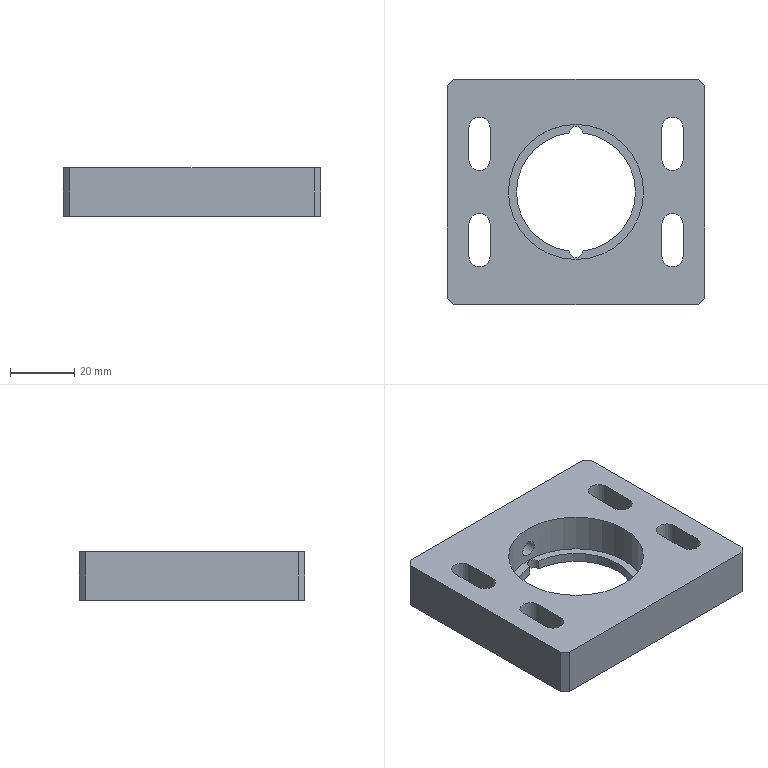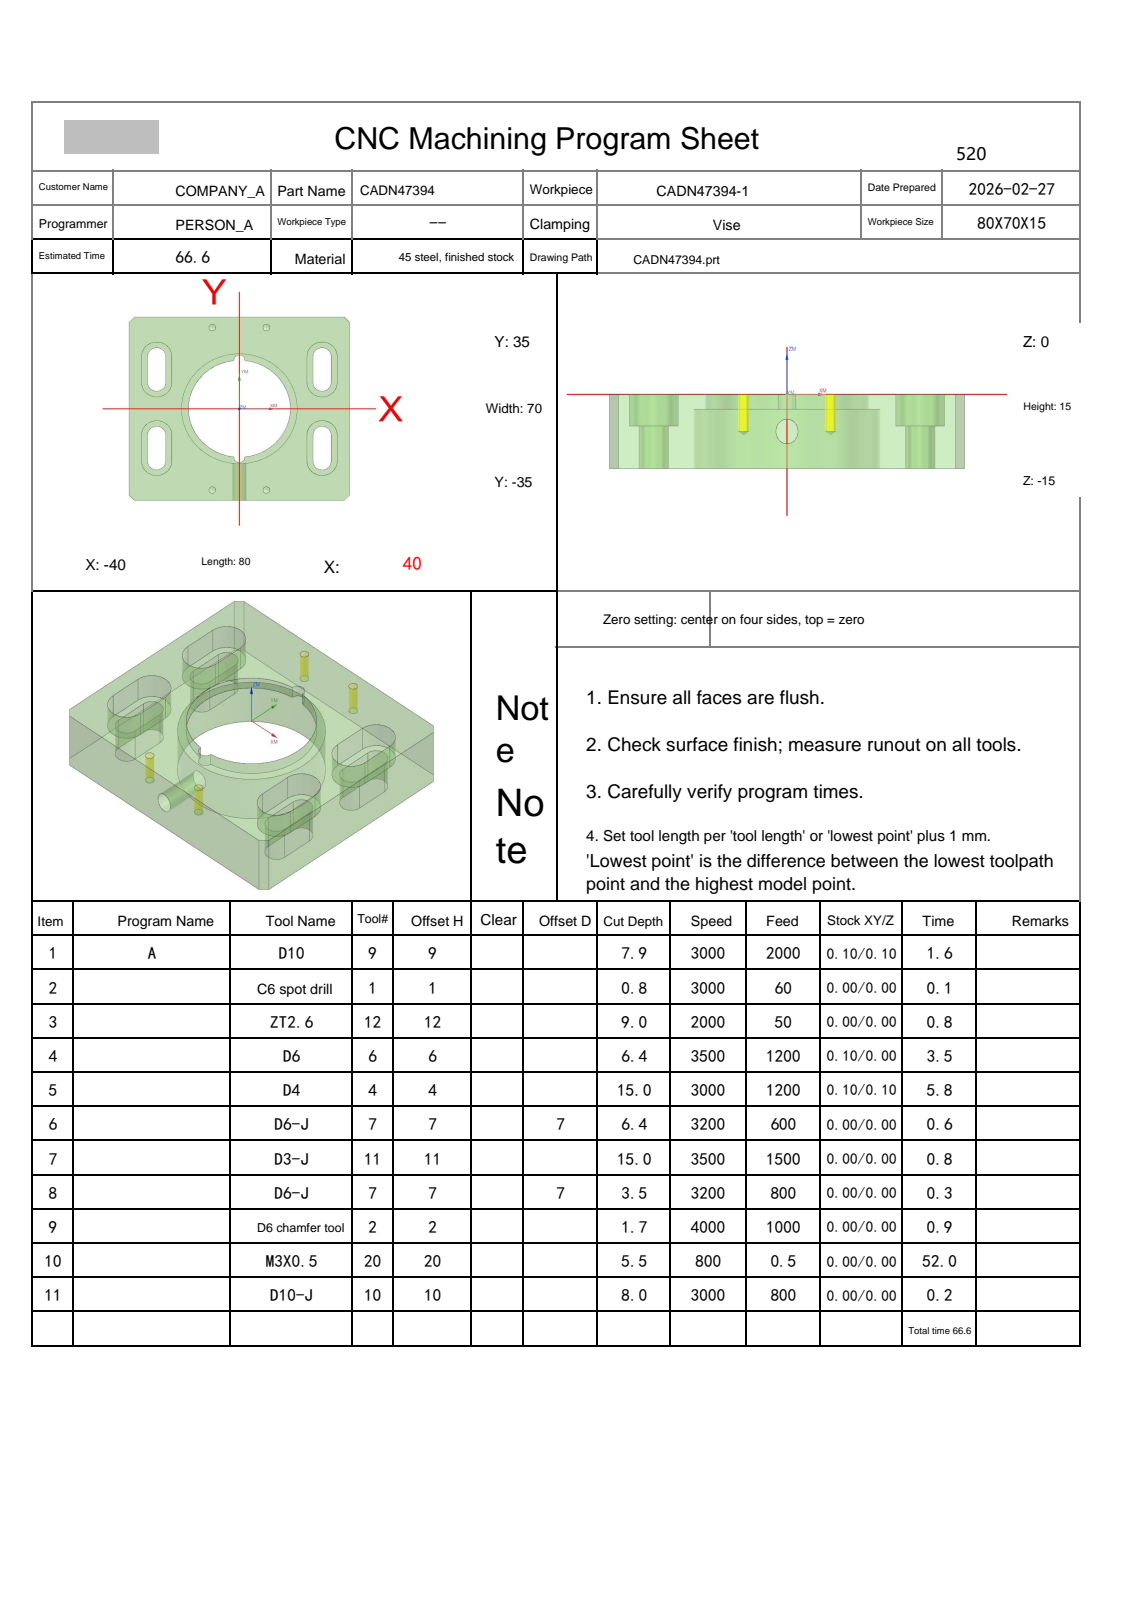NC program | NX | posted by the shop | part box 80 x 70 x 15 mm
Lines 3270 to 4817 of 4817:
N7 T11 M06
(D3-J  D=3. R=0. H=11 ce=0.00 di=0.01)
G00 G90 G54 X2.541 Y15.76 M03 S3500
G43 H11 Z50.
M08
Z.2
G01 X2.538 Y15.772 Z.116 F1200.
X2.53 Y15.806 Z.042
X2.514 Y15.861 Z-.022
X2.488 Y15.933 Z-.077
X2.449 Y16.022 Z-.122
X2.397 Y16.125 Z-.16
X2.329 Y16.24 Z-.19
X2.243 Y16.366 Z-.213
X2.137 Y16.499 Z-.23
X2.009 Y16.638 Z-.242
X1.858 Y16.781 Z-.248
X1.68 Y16.926 Z-.25
G02 X.497 Y18.392 I.317 J1.466 F1500.
G01 X.499 Y18.473
X.5 Y18.5
G03 X0.0 Y19. I-.5 J0.0
X-.5 Y18.5 I0.0 J-.5
G01 X-.499 Y18.473
X-.497 Y18.392
G02 X-1.68 Y16.926 I-1.5 J0.0
G01 X-1.798 Y16.894 Z-.251
X-1.88 Y16.857 Z-.252
X-1.931 Y16.817 Z-.255
X-1.952 Y16.773 Z-.258
X-1.944 Y16.727 Z-.262
X-1.911 Y16.68 Z-.267
X-1.855 Y16.631 Z-.273
X-1.777 Y16.583 Z-.279
X-1.679 Y16.536 Z-.286
X-1.565 Y16.491 Z-.294
X-1.435 Y16.448 Z-.301
X-1.293 Y16.409 Z-.309
X-1.14 Y16.374 Z-.318
X-.782 Y16.315 Z-.336
X-.397 Y16.28 Z-.356
X.001 Y16.268 Z-.375
X.399 Y16.279 Z-.394
X.783 Y16.315 Z-.414
X1.142 Y16.374 Z-.432
X1.294 Y16.409 Z-.441
X1.436 Y16.448 Z-.449
X1.566 Y16.491 Z-.456
X1.68 Y16.536 Z-.464
X1.777 Y16.583 Z-.471
X1.855 Y16.631 Z-.477
X1.912 Y16.679 Z-.483
X1.945 Y16.727 Z-.488
X1.952 Y16.773 Z-.492
X1.931 Y16.817 Z-.495
X1.881 Y16.857 Z-.498
X1.798 Y16.894 Z-.499
X1.68 Y16.926 Z-.5
G02 X.497 Y18.392 I.317 J1.466
G01 X.499 Y18.473
X.5 Y18.5
G03 X0.0 Y19. I-.5 J0.0
X-.5 Y18.5 I0.0 J-.5
G01 X-.499 Y18.473
X-.497 Y18.392
G02 X-1.68 Y16.926 I-1.5 J0.0
G01 X-1.798 Y16.894 Z-.501
X-1.88 Y16.857 Z-.502
X-1.931 Y16.817 Z-.505
X-1.952 Y16.773 Z-.508
X-1.944 Y16.727 Z-.512
X-1.911 Y16.68 Z-.517
X-1.855 Y16.631 Z-.523
X-1.777 Y16.583 Z-.529
X-1.679 Y16.536 Z-.536
X-1.565 Y16.491 Z-.544
X-1.435 Y16.448 Z-.551
X-1.293 Y16.409 Z-.559
X-1.14 Y16.374 Z-.568
X-.782 Y16.315 Z-.586
X-.397 Y16.28 Z-.606
X.001 Y16.268 Z-.625
X.399 Y16.279 Z-.644
X.783 Y16.315 Z-.664
X1.142 Y16.374 Z-.682
X1.294 Y16.409 Z-.691
X1.436 Y16.448 Z-.699
X1.566 Y16.491 Z-.706
X1.68 Y16.536 Z-.714
X1.777 Y16.583 Z-.721
X1.855 Y16.631 Z-.727
X1.912 Y16.679 Z-.733
X1.945 Y16.727 Z-.738
X1.952 Y16.773 Z-.742
X1.931 Y16.817 Z-.745
X1.881 Y16.857 Z-.748
X1.798 Y16.894 Z-.749
X1.68 Y16.926 Z-.75
G02 X.497 Y18.392 I.317 J1.466
G01 X.499 Y18.473
X.5 Y18.5
G03 X0.0 Y19. I-.5 J0.0
X-.5 Y18.5 I0.0 J-.5
G01 X-.499 Y18.473
X-.497 Y18.392
G02 X-1.68 Y16.926 I-1.5 J0.0
G01 X-1.798 Y16.894 Z-.751
X-1.88 Y16.857 Z-.752
X-1.931 Y16.817 Z-.755
X-1.952 Y16.773 Z-.758
X-1.944 Y16.727 Z-.762
X-1.911 Y16.68 Z-.767
X-1.855 Y16.631 Z-.773
X-1.777 Y16.583 Z-.779
X-1.679 Y16.536 Z-.786
X-1.565 Y16.491 Z-.794
X-1.435 Y16.448 Z-.801
X-1.293 Y16.409 Z-.809
X-1.14 Y16.374 Z-.818
X-.782 Y16.315 Z-.836
X-.397 Y16.28 Z-.856
X.001 Y16.268 Z-.875
X.399 Y16.279 Z-.894
X.783 Y16.315 Z-.914
X1.142 Y16.374 Z-.932
X1.294 Y16.409 Z-.941
X1.436 Y16.448 Z-.949
X1.566 Y16.491 Z-.956
X1.68 Y16.536 Z-.964
X1.777 Y16.583 Z-.971
X1.855 Y16.631 Z-.977
X1.912 Y16.679 Z-.983
X1.945 Y16.727 Z-.988
X1.952 Y16.773 Z-.992
X1.931 Y16.817 Z-.995
X1.881 Y16.857 Z-.998
X1.798 Y16.894 Z-.999
X1.68 Y16.926 Z-1.
G02 X.497 Y18.392 I.317 J1.466
G01 X.499 Y18.473
X.5 Y18.5
G03 X0.0 Y19. I-.5 J0.0
X-.5 Y18.5 I0.0 J-.5
G01 X-.499 Y18.473
X-.497 Y18.392
G02 X-1.68 Y16.926 I-1.5 J0.0
G01 X-1.798 Y16.894 Z-1.001
X-1.88 Y16.857 Z-1.002
X-1.931 Y16.817 Z-1.005
X-1.952 Y16.773 Z-1.008
X-1.944 Y16.727 Z-1.012
X-1.911 Y16.68 Z-1.017
X-1.855 Y16.631 Z-1.023
X-1.777 Y16.583 Z-1.029
X-1.679 Y16.536 Z-1.036
X-1.565 Y16.491 Z-1.044
X-1.435 Y16.448 Z-1.051
X-1.293 Y16.409 Z-1.059
X-1.14 Y16.374 Z-1.068
X-.782 Y16.315 Z-1.086
X-.397 Y16.28 Z-1.106
X.001 Y16.268 Z-1.125
X.399 Y16.279 Z-1.144
X.783 Y16.315 Z-1.164
X1.142 Y16.374 Z-1.182
X1.294 Y16.409 Z-1.191
X1.436 Y16.448 Z-1.199
X1.566 Y16.491 Z-1.206
X1.68 Y16.536 Z-1.214
X1.777 Y16.583 Z-1.221
X1.855 Y16.631 Z-1.227
X1.912 Y16.679 Z-1.233
X1.945 Y16.727 Z-1.238
X1.952 Y16.773 Z-1.242
X1.931 Y16.817 Z-1.245
X1.881 Y16.857 Z-1.248
X1.798 Y16.894 Z-1.249
X1.68 Y16.926 Z-1.25
G02 X.497 Y18.392 I.317 J1.466
G01 X.499 Y18.473
X.5 Y18.5
G03 X0.0 Y19. I-.5 J0.0
X-.5 Y18.5 I0.0 J-.5
G01 X-.499 Y18.473
X-.497 Y18.392
G02 X-1.68 Y16.926 I-1.5 J0.0
G01 X-1.798 Y16.894 Z-1.251
X-1.88 Y16.857 Z-1.252
X-1.931 Y16.817 Z-1.255
X-1.952 Y16.773 Z-1.258
X-1.944 Y16.727 Z-1.262
X-1.911 Y16.68 Z-1.267
X-1.855 Y16.631 Z-1.273
X-1.777 Y16.583 Z-1.279
X-1.679 Y16.536 Z-1.286
X-1.565 Y16.491 Z-1.294
X-1.435 Y16.448 Z-1.301
X-1.293 Y16.409 Z-1.309
X-1.14 Y16.374 Z-1.318
X-.782 Y16.315 Z-1.336
X-.397 Y16.28 Z-1.356
X.001 Y16.268 Z-1.375
X.399 Y16.279 Z-1.394
X.783 Y16.315 Z-1.414
X1.142 Y16.374 Z-1.432
X1.294 Y16.409 Z-1.441
X1.436 Y16.448 Z-1.449
X1.566 Y16.491 Z-1.456
X1.68 Y16.536 Z-1.464
X1.777 Y16.583 Z-1.471
X1.855 Y16.631 Z-1.477
X1.912 Y16.679 Z-1.483
X1.945 Y16.727 Z-1.488
X1.952 Y16.773 Z-1.492
X1.931 Y16.817 Z-1.495
X1.881 Y16.857 Z-1.498
X1.798 Y16.894 Z-1.499
X1.68 Y16.926 Z-1.5
G02 X.497 Y18.392 I.317 J1.466
G01 X.499 Y18.473
X.5 Y18.5
G03 X0.0 Y19. I-.5 J0.0
X-.5 Y18.5 I0.0 J-.5
G01 X-.499 Y18.473
X-.497 Y18.392
G02 X-1.68 Y16.926 I-1.5 J0.0
G01 X-1.798 Y16.894 Z-1.501
X-1.88 Y16.857 Z-1.502
X-1.931 Y16.817 Z-1.505
X-1.952 Y16.773 Z-1.508
X-1.944 Y16.727 Z-1.512
X-1.911 Y16.68 Z-1.517
X-1.855 Y16.631 Z-1.523
X-1.777 Y16.583 Z-1.529
X-1.679 Y16.536 Z-1.536
X-1.565 Y16.491 Z-1.544
X-1.435 Y16.448 Z-1.551
X-1.293 Y16.409 Z-1.559
X-1.14 Y16.374 Z-1.568
X-.782 Y16.315 Z-1.586
X-.397 Y16.28 Z-1.606
X.001 Y16.268 Z-1.625
X.399 Y16.279 Z-1.644
X.783 Y16.315 Z-1.664
X1.142 Y16.374 Z-1.682
X1.294 Y16.409 Z-1.691
X1.436 Y16.448 Z-1.699
X1.566 Y16.491 Z-1.706
X1.68 Y16.536 Z-1.714
X1.777 Y16.583 Z-1.721
X1.855 Y16.631 Z-1.727
X1.912 Y16.679 Z-1.733
X1.945 Y16.727 Z-1.738
X1.952 Y16.773 Z-1.742
X1.931 Y16.817 Z-1.745
X1.881 Y16.857 Z-1.748
X1.798 Y16.894 Z-1.749
X1.68 Y16.926 Z-1.75
G02 X.497 Y18.392 I.317 J1.466
G01 X.499 Y18.473
X.5 Y18.5
G03 X0.0 Y19. I-.5 J0.0
X-.5 Y18.5 I0.0 J-.5
G01 X-.499 Y18.473
X-.497 Y18.392
G02 X-1.68 Y16.926 I-1.5 J0.0
G01 X-1.798 Y16.894 Z-1.751
X-1.88 Y16.857 Z-1.752
X-1.931 Y16.817 Z-1.755
X-1.952 Y16.773 Z-1.758
X-1.944 Y16.727 Z-1.762
X-1.911 Y16.68 Z-1.767
X-1.855 Y16.631 Z-1.773
X-1.777 Y16.583 Z-1.779
X-1.679 Y16.536 Z-1.786
X-1.565 Y16.491 Z-1.794
X-1.435 Y16.448 Z-1.801
X-1.293 Y16.409 Z-1.809
X-1.14 Y16.374 Z-1.818
X-.782 Y16.315 Z-1.836
X-.397 Y16.28 Z-1.856
X.001 Y16.268 Z-1.875
X.399 Y16.279 Z-1.894
X.783 Y16.315 Z-1.914
X1.142 Y16.374 Z-1.932
X1.294 Y16.409 Z-1.941
X1.436 Y16.448 Z-1.949
X1.566 Y16.491 Z-1.956
X1.68 Y16.536 Z-1.964
X1.777 Y16.583 Z-1.971
X1.855 Y16.631 Z-1.977
X1.912 Y16.679 Z-1.983
X1.945 Y16.727 Z-1.988
X1.952 Y16.773 Z-1.992
X1.931 Y16.817 Z-1.995
X1.881 Y16.857 Z-1.998
X1.798 Y16.894 Z-1.999
X1.68 Y16.926 Z-2.
G02 X.497 Y18.392 I.317 J1.466
G01 X.499 Y18.473
X.5 Y18.5
G03 X0.0 Y19. I-.5 J0.0
X-.5 Y18.5 I0.0 J-.5
G01 X-.499 Y18.473
X-.497 Y18.392
G02 X-1.68 Y16.926 I-1.5 J0.0
G01 X-1.798 Y16.894 Z-2.001
X-1.88 Y16.857 Z-2.002
X-1.931 Y16.817 Z-2.005
X-1.952 Y16.773 Z-2.008
X-1.944 Y16.727 Z-2.012
X-1.911 Y16.68 Z-2.017
X-1.855 Y16.631 Z-2.023
X-1.777 Y16.583 Z-2.029
X-1.679 Y16.536 Z-2.036
X-1.565 Y16.491 Z-2.044
X-1.435 Y16.448 Z-2.051
X-1.293 Y16.409 Z-2.059
X-1.14 Y16.374 Z-2.068
X-.782 Y16.315 Z-2.086
X-.397 Y16.28 Z-2.106
X.001 Y16.268 Z-2.125
X.399 Y16.279 Z-2.144
X.783 Y16.315 Z-2.164
X1.142 Y16.374 Z-2.182
X1.294 Y16.409 Z-2.191
X1.436 Y16.448 Z-2.199
X1.566 Y16.491 Z-2.206
X1.68 Y16.536 Z-2.214
X1.777 Y16.583 Z-2.221
X1.855 Y16.631 Z-2.227
X1.912 Y16.679 Z-2.233
X1.945 Y16.727 Z-2.238
X1.952 Y16.773 Z-2.242
X1.931 Y16.817 Z-2.245
X1.881 Y16.857 Z-2.248
X1.798 Y16.894 Z-2.249
X1.68 Y16.926 Z-2.25
G02 X.497 Y18.392 I.317 J1.466
G01 X.499 Y18.473
X.5 Y18.5
G03 X0.0 Y19. I-.5 J0.0
X-.5 Y18.5 I0.0 J-.5
G01 X-.499 Y18.473
X-.497 Y18.392
G02 X-1.68 Y16.926 I-1.5 J0.0
G01 X-1.798 Y16.894 Z-2.251
X-1.88 Y16.857 Z-2.252
X-1.931 Y16.817 Z-2.255
X-1.952 Y16.773 Z-2.258
X-1.944 Y16.727 Z-2.262
X-1.911 Y16.68 Z-2.267
X-1.855 Y16.631 Z-2.273
X-1.777 Y16.583 Z-2.279
X-1.679 Y16.536 Z-2.286
X-1.565 Y16.491 Z-2.294
X-1.435 Y16.448 Z-2.301
X-1.293 Y16.409 Z-2.309
X-1.14 Y16.374 Z-2.318
X-.782 Y16.315 Z-2.336
X-.397 Y16.28 Z-2.356
X.001 Y16.268 Z-2.375
X.399 Y16.279 Z-2.394
X.783 Y16.315 Z-2.414
X1.142 Y16.374 Z-2.432
X1.294 Y16.409 Z-2.441
X1.436 Y16.448 Z-2.449
X1.566 Y16.491 Z-2.456
X1.68 Y16.536 Z-2.464
X1.777 Y16.583 Z-2.471
X1.855 Y16.631 Z-2.477
X1.912 Y16.679 Z-2.483
X1.945 Y16.727 Z-2.488
X1.952 Y16.773 Z-2.492
X1.931 Y16.817 Z-2.495
X1.881 Y16.857 Z-2.498
X1.798 Y16.894 Z-2.499
X1.68 Y16.926 Z-2.5
G02 X.497 Y18.392 I.317 J1.466
G01 X.499 Y18.473
X.5 Y18.5
G03 X0.0 Y19. I-.5 J0.0
X-.5 Y18.5 I0.0 J-.5
G01 X-.499 Y18.473
X-.497 Y18.392
G02 X-1.68 Y16.926 I-1.5 J0.0
G01 X-1.798 Y16.894 Z-2.501
X-1.88 Y16.857 Z-2.502
X-1.931 Y16.817 Z-2.505
X-1.952 Y16.773 Z-2.508
X-1.944 Y16.727 Z-2.512
X-1.911 Y16.68 Z-2.517
X-1.855 Y16.631 Z-2.523
X-1.777 Y16.583 Z-2.529
X-1.679 Y16.536 Z-2.536
X-1.565 Y16.491 Z-2.544
X-1.435 Y16.448 Z-2.551
X-1.293 Y16.409 Z-2.559
X-1.14 Y16.374 Z-2.568
X-.782 Y16.315 Z-2.586
X-.397 Y16.28 Z-2.606
X.001 Y16.268 Z-2.625
X.399 Y16.279 Z-2.644
X.783 Y16.315 Z-2.664
X1.142 Y16.374 Z-2.682
X1.294 Y16.409 Z-2.691
X1.436 Y16.448 Z-2.699
X1.566 Y16.491 Z-2.706
X1.68 Y16.536 Z-2.714
X1.777 Y16.583 Z-2.721
X1.855 Y16.631 Z-2.727
X1.912 Y16.679 Z-2.733
X1.945 Y16.727 Z-2.738
X1.952 Y16.773 Z-2.742
X1.931 Y16.817 Z-2.745
X1.881 Y16.857 Z-2.748
X1.798 Y16.894 Z-2.749
X1.68 Y16.926 Z-2.75
G02 X.497 Y18.392 I.317 J1.466
G01 X.499 Y18.473
X.5 Y18.5
G03 X0.0 Y19. I-.5 J0.0
X-.5 Y18.5 I0.0 J-.5
G01 X-.499 Y18.473
X-.497 Y18.392
G02 X-1.68 Y16.926 I-1.5 J0.0
G01 X-1.798 Y16.894 Z-2.751
X-1.88 Y16.857 Z-2.752
X-1.931 Y16.817 Z-2.755
X-1.952 Y16.773 Z-2.758
X-1.944 Y16.727 Z-2.762
X-1.911 Y16.68 Z-2.767
X-1.855 Y16.631 Z-2.773
X-1.777 Y16.583 Z-2.779
X-1.679 Y16.536 Z-2.786
X-1.565 Y16.491 Z-2.794
X-1.435 Y16.448 Z-2.801
X-1.293 Y16.409 Z-2.809
X-1.14 Y16.374 Z-2.818
X-.782 Y16.315 Z-2.836
X-.397 Y16.28 Z-2.856
X.001 Y16.268 Z-2.875
X.399 Y16.279 Z-2.894
X.783 Y16.315 Z-2.914
X1.142 Y16.374 Z-2.932
X1.294 Y16.409 Z-2.941
X1.436 Y16.448 Z-2.949
X1.566 Y16.491 Z-2.956
X1.68 Y16.536 Z-2.964
X1.777 Y16.583 Z-2.971
X1.855 Y16.631 Z-2.977
X1.912 Y16.679 Z-2.983
X1.945 Y16.727 Z-2.988
X1.952 Y16.773 Z-2.992
X1.931 Y16.817 Z-2.995
X1.881 Y16.857 Z-2.998
X1.798 Y16.894 Z-2.999
X1.68 Y16.926 Z-3.
G02 X.497 Y18.392 I.317 J1.466
G01 X.499 Y18.473
X.5 Y18.5
G03 X0.0 Y19. I-.5 J0.0
X-.5 Y18.5 I0.0 J-.5
G01 X-.499 Y18.473
X-.497 Y18.392
G02 X-1.68 Y16.926 I-1.5 J0.0
G01 X-1.798 Y16.894 Z-3.001
X-1.88 Y16.857 Z-3.002
X-1.931 Y16.817 Z-3.005
X-1.952 Y16.773 Z-3.008
X-1.944 Y16.727 Z-3.012
X-1.911 Y16.68 Z-3.017
X-1.855 Y16.631 Z-3.023
X-1.777 Y16.583 Z-3.029
X-1.679 Y16.536 Z-3.036
X-1.565 Y16.491 Z-3.044
X-1.435 Y16.448 Z-3.051
X-1.293 Y16.409 Z-3.059
X-1.14 Y16.374 Z-3.068
X-.782 Y16.315 Z-3.086
X-.397 Y16.28 Z-3.106
X.001 Y16.268 Z-3.125
X.399 Y16.279 Z-3.144
X.783 Y16.315 Z-3.164
X1.142 Y16.374 Z-3.182
X1.294 Y16.409 Z-3.191
X1.436 Y16.448 Z-3.199
X1.566 Y16.491 Z-3.206
X1.68 Y16.536 Z-3.214
X1.777 Y16.583 Z-3.221
X1.855 Y16.631 Z-3.227
X1.912 Y16.679 Z-3.233
X1.945 Y16.727 Z-3.238
X1.952 Y16.773 Z-3.242
X1.931 Y16.817 Z-3.245
X1.881 Y16.857 Z-3.248
X1.798 Y16.894 Z-3.249
X1.68 Y16.926 Z-3.25
G02 X.497 Y18.392 I.317 J1.466
G01 X.499 Y18.473
X.5 Y18.5
G03 X0.0 Y19. I-.5 J0.0
X-.5 Y18.5 I0.0 J-.5
G01 X-.499 Y18.473
X-.497 Y18.392
G02 X-1.68 Y16.926 I-1.5 J0.0
G01 X-1.798 Y16.894 Z-3.251
X-1.88 Y16.857 Z-3.252
X-1.931 Y16.817 Z-3.255
X-1.952 Y16.773 Z-3.258
X-1.944 Y16.727 Z-3.262
X-1.911 Y16.68 Z-3.267
X-1.855 Y16.631 Z-3.273
X-1.777 Y16.583 Z-3.279
X-1.679 Y16.536 Z-3.286
X-1.565 Y16.491 Z-3.294
X-1.435 Y16.448 Z-3.301
X-1.293 Y16.409 Z-3.309
X-1.14 Y16.374 Z-3.318
X-.782 Y16.315 Z-3.336
X-.397 Y16.28 Z-3.356
X.001 Y16.268 Z-3.375
X.399 Y16.279 Z-3.394
X.783 Y16.315 Z-3.414
X1.142 Y16.374 Z-3.432
X1.294 Y16.409 Z-3.441
X1.436 Y16.448 Z-3.449
X1.566 Y16.491 Z-3.456
X1.68 Y16.536 Z-3.464
X1.777 Y16.583 Z-3.471
X1.855 Y16.631 Z-3.477
X1.912 Y16.679 Z-3.483
X1.945 Y16.727 Z-3.488
X1.952 Y16.773 Z-3.492
X1.931 Y16.817 Z-3.495
X1.881 Y16.857 Z-3.498
X1.798 Y16.894 Z-3.499
X1.68 Y16.926 Z-3.5
G02 X.497 Y18.392 I.317 J1.466
G01 X.499 Y18.473
X.5 Y18.5
G03 X0.0 Y19. I-.5 J0.0
X-.5 Y18.5 I0.0 J-.5
G01 X-.499 Y18.473
X-.497 Y18.392
G02 X-1.68 Y16.926 I-1.5 J0.0
G01 X-1.858 Y16.781 Z-3.498
X-2.009 Y16.638 Z-3.492
X-2.137 Y16.499 Z-3.48
X-2.243 Y16.366 Z-3.463
X-2.329 Y16.241 Z-3.44
X-2.396 Y16.126 Z-3.41
X-2.448 Y16.023 Z-3.372
X-2.487 Y15.934 Z-3.327
X-2.513 Y15.861 Z-3.272
X-2.529 Y15.807 Z-3.208
X-2.537 Y15.772 Z-3.134
X-2.539 Y15.761 Z-3.05
G00 Z50.
X-2.541 Y-15.76
Z.2
G01 X-2.538 Y-15.772 Z.116 F1200.
X-2.53 Y-15.806 Z.042
X-2.514 Y-15.861 Z-.022
X-2.488 Y-15.933 Z-.077
X-2.449 Y-16.022 Z-.122
X-2.397 Y-16.125 Z-.16
X-2.329 Y-16.24 Z-.19
X-2.243 Y-16.366 Z-.213
X-2.137 Y-16.499 Z-.23
X-2.009 Y-16.638 Z-.242
X-1.858 Y-16.781 Z-.248
X-1.68 Y-16.926 Z-.25
G02 X-.497 Y-18.392 I-.317 J-1.466 F1500.
G01 X-.499 Y-18.473
X-.5 Y-18.5
G03 X0.0 Y-19. I.5 J0.0
X.5 Y-18.5 I0.0 J.5
G01 X.499 Y-18.473
X.497 Y-18.392
G02 X1.68 Y-16.926 I1.5 J0.0
G01 X1.798 Y-16.894 Z-.251
X1.881 Y-16.857 Z-.252
X1.931 Y-16.817 Z-.255
X1.952 Y-16.773 Z-.258
X1.945 Y-16.727 Z-.262
X1.912 Y-16.679 Z-.267
X1.855 Y-16.631 Z-.273
X1.777 Y-16.583 Z-.279
X1.68 Y-16.536 Z-.286
X1.565 Y-16.491 Z-.294
X1.436 Y-16.448 Z-.301
X1.294 Y-16.409 Z-.309
X1.141 Y-16.374 Z-.318
X.783 Y-16.315 Z-.336
X.398 Y-16.279 Z-.356
X0.0 Y-16.268 Z-.375
X-.398 Y-16.279 Z-.394
X-.783 Y-16.315 Z-.414
X-1.141 Y-16.374 Z-.432
X-1.294 Y-16.409 Z-.441
X-1.436 Y-16.448 Z-.449
X-1.565 Y-16.491 Z-.456
X-1.68 Y-16.536 Z-.464
X-1.777 Y-16.583 Z-.471
X-1.855 Y-16.631 Z-.477
X-1.912 Y-16.679 Z-.483
X-1.945 Y-16.727 Z-.488
X-1.952 Y-16.773 Z-.492
X-1.931 Y-16.817 Z-.495
X-1.881 Y-16.857 Z-.498
X-1.798 Y-16.894 Z-.499
X-1.68 Y-16.926 Z-.5
G02 X-.497 Y-18.392 I-.317 J-1.466
G01 X-.499 Y-18.473
X-.5 Y-18.5
G03 X0.0 Y-19. I.5 J0.0
X.5 Y-18.5 I0.0 J.5
G01 X.499 Y-18.473
X.497 Y-18.392
G02 X1.68 Y-16.926 I1.5 J0.0
G01 X1.798 Y-16.894 Z-.501
X1.881 Y-16.857 Z-.502
X1.931 Y-16.817 Z-.505
X1.952 Y-16.773 Z-.508
X1.945 Y-16.727 Z-.512
X1.912 Y-16.679 Z-.517
X1.855 Y-16.631 Z-.523
X1.777 Y-16.583 Z-.529
X1.68 Y-16.536 Z-.536
X1.565 Y-16.491 Z-.544
X1.436 Y-16.448 Z-.551
X1.294 Y-16.409 Z-.559
X1.141 Y-16.374 Z-.568
X.783 Y-16.315 Z-.586
X.398 Y-16.279 Z-.606
X0.0 Y-16.268 Z-.625
X-.398 Y-16.279 Z-.644
X-.783 Y-16.315 Z-.664
X-1.141 Y-16.374 Z-.682
X-1.294 Y-16.409 Z-.691
X-1.436 Y-16.448 Z-.699
X-1.565 Y-16.491 Z-.706
X-1.68 Y-16.536 Z-.714
X-1.777 Y-16.583 Z-.721
X-1.855 Y-16.631 Z-.727
X-1.912 Y-16.679 Z-.733
X-1.945 Y-16.727 Z-.738
X-1.952 Y-16.773 Z-.742
X-1.931 Y-16.817 Z-.745
X-1.881 Y-16.857 Z-.748
X-1.798 Y-16.894 Z-.749
X-1.68 Y-16.926 Z-.75
G02 X-.497 Y-18.392 I-.317 J-1.466
G01 X-.499 Y-18.473
X-.5 Y-18.5
G03 X0.0 Y-19. I.5 J0.0
X.5 Y-18.5 I0.0 J.5
G01 X.499 Y-18.473
X.497 Y-18.392
G02 X1.68 Y-16.926 I1.5 J0.0
G01 X1.798 Y-16.894 Z-.751
X1.881 Y-16.857 Z-.752
X1.931 Y-16.817 Z-.755
X1.952 Y-16.773 Z-.758
X1.945 Y-16.727 Z-.762
X1.912 Y-16.679 Z-.767
X1.855 Y-16.631 Z-.773
X1.777 Y-16.583 Z-.779
X1.68 Y-16.536 Z-.786
X1.565 Y-16.491 Z-.794
X1.436 Y-16.448 Z-.801
X1.294 Y-16.409 Z-.809
X1.141 Y-16.374 Z-.818
X.783 Y-16.315 Z-.836
X.398 Y-16.279 Z-.856
X0.0 Y-16.268 Z-.875
X-.398 Y-16.279 Z-.894
X-.783 Y-16.315 Z-.914
X-1.141 Y-16.374 Z-.932
X-1.294 Y-16.409 Z-.941
X-1.436 Y-16.448 Z-.949
X-1.565 Y-16.491 Z-.956
X-1.68 Y-16.536 Z-.964
X-1.777 Y-16.583 Z-.971
X-1.855 Y-16.631 Z-.977
X-1.912 Y-16.679 Z-.983
X-1.945 Y-16.727 Z-.988
X-1.952 Y-16.773 Z-.992
X-1.931 Y-16.817 Z-.995
X-1.881 Y-16.857 Z-.998
X-1.798 Y-16.894 Z-.999
X-1.68 Y-16.926 Z-1.
G02 X-.497 Y-18.392 I-.317 J-1.466
G01 X-.499 Y-18.473
X-.5 Y-18.5
G03 X0.0 Y-19. I.5 J0.0
X.5 Y-18.5 I0.0 J.5
G01 X.499 Y-18.473
X.497 Y-18.392
G02 X1.68 Y-16.926 I1.5 J0.0
G01 X1.798 Y-16.894 Z-1.001
X1.881 Y-16.857 Z-1.002
X1.931 Y-16.817 Z-1.005
X1.952 Y-16.773 Z-1.008
X1.945 Y-16.727 Z-1.012
X1.912 Y-16.679 Z-1.017
X1.855 Y-16.631 Z-1.023
X1.777 Y-16.583 Z-1.029
X1.68 Y-16.536 Z-1.036
X1.565 Y-16.491 Z-1.044
X1.436 Y-16.448 Z-1.051
X1.294 Y-16.409 Z-1.059
X1.141 Y-16.374 Z-1.068
X.783 Y-16.315 Z-1.086
X.398 Y-16.279 Z-1.106
X0.0 Y-16.268 Z-1.125
X-.398 Y-16.279 Z-1.144
X-.783 Y-16.315 Z-1.164
X-1.141 Y-16.374 Z-1.182
X-1.294 Y-16.409 Z-1.191
X-1.436 Y-16.448 Z-1.199
X-1.565 Y-16.491 Z-1.206
X-1.68 Y-16.536 Z-1.214
X-1.777 Y-16.583 Z-1.221
X-1.855 Y-16.631 Z-1.227
X-1.912 Y-16.679 Z-1.233
X-1.945 Y-16.727 Z-1.238
X-1.952 Y-16.773 Z-1.242
X-1.931 Y-16.817 Z-1.245
X-1.881 Y-16.857 Z-1.248
X-1.798 Y-16.894 Z-1.249
X-1.68 Y-16.926 Z-1.25
G02 X-.497 Y-18.392 I-.317 J-1.466
G01 X-.499 Y-18.473
X-.5 Y-18.5
G03 X0.0 Y-19. I.5 J0.0
X.5 Y-18.5 I0.0 J.5
G01 X.499 Y-18.473
X.497 Y-18.392
G02 X1.68 Y-16.926 I1.5 J0.0
G01 X1.798 Y-16.894 Z-1.251
X1.881 Y-16.857 Z-1.252
X1.931 Y-16.817 Z-1.255
X1.952 Y-16.773 Z-1.258
X1.945 Y-16.727 Z-1.262
X1.912 Y-16.679 Z-1.267
X1.855 Y-16.631 Z-1.273
X1.777 Y-16.583 Z-1.279
X1.68 Y-16.536 Z-1.286
X1.565 Y-16.491 Z-1.294
X1.436 Y-16.448 Z-1.301
X1.294 Y-16.409 Z-1.309
X1.141 Y-16.374 Z-1.318
X.783 Y-16.315 Z-1.336
X.398 Y-16.279 Z-1.356
X0.0 Y-16.268 Z-1.375
X-.398 Y-16.279 Z-1.394
X-.783 Y-16.315 Z-1.414
X-1.141 Y-16.374 Z-1.432
X-1.294 Y-16.409 Z-1.441
X-1.436 Y-16.448 Z-1.449
X-1.565 Y-16.491 Z-1.456
X-1.68 Y-16.536 Z-1.464
X-1.777 Y-16.583 Z-1.471
X-1.855 Y-16.631 Z-1.477
X-1.912 Y-16.679 Z-1.483
X-1.945 Y-16.727 Z-1.488
X-1.952 Y-16.773 Z-1.492
X-1.931 Y-16.817 Z-1.495
X-1.881 Y-16.857 Z-1.498
X-1.798 Y-16.894 Z-1.499
X-1.68 Y-16.926 Z-1.5
G02 X-.497 Y-18.392 I-.317 J-1.466
G01 X-.499 Y-18.473
X-.5 Y-18.5
G03 X0.0 Y-19. I.5 J0.0
X.5 Y-18.5 I0.0 J.5
G01 X.499 Y-18.473
X.497 Y-18.392
G02 X1.68 Y-16.926 I1.5 J0.0
G01 X1.798 Y-16.894 Z-1.501
X1.881 Y-16.857 Z-1.502
X1.931 Y-16.817 Z-1.505
X1.952 Y-16.773 Z-1.508
X1.945 Y-16.727 Z-1.512
X1.912 Y-16.679 Z-1.517
X1.855 Y-16.631 Z-1.523
X1.777 Y-16.583 Z-1.529
X1.68 Y-16.536 Z-1.536
X1.565 Y-16.491 Z-1.544
X1.436 Y-16.448 Z-1.551
X1.294 Y-16.409 Z-1.559
X1.141 Y-16.374 Z-1.568
X.783 Y-16.315 Z-1.586
X.398 Y-16.279 Z-1.606
X0.0 Y-16.268 Z-1.625
X-.398 Y-16.279 Z-1.644
X-.783 Y-16.315 Z-1.664
X-1.141 Y-16.374 Z-1.682
X-1.294 Y-16.409 Z-1.691
X-1.436 Y-16.448 Z-1.699
X-1.565 Y-16.491 Z-1.706
X-1.68 Y-16.536 Z-1.714
X-1.777 Y-16.583 Z-1.721
X-1.855 Y-16.631 Z-1.727
X-1.912 Y-16.679 Z-1.733
X-1.945 Y-16.727 Z-1.738
X-1.952 Y-16.773 Z-1.742
X-1.931 Y-16.817 Z-1.745
X-1.881 Y-16.857 Z-1.748
X-1.798 Y-16.894 Z-1.749
X-1.68 Y-16.926 Z-1.75
G02 X-.497 Y-18.392 I-.317 J-1.466
G01 X-.499 Y-18.473
X-.5 Y-18.5
G03 X0.0 Y-19. I.5 J0.0
X.5 Y-18.5 I0.0 J.5
G01 X.499 Y-18.473
X.497 Y-18.392
G02 X1.68 Y-16.926 I1.5 J0.0
G01 X1.798 Y-16.894 Z-1.751
X1.881 Y-16.857 Z-1.752
X1.931 Y-16.817 Z-1.755
X1.952 Y-16.773 Z-1.758
X1.945 Y-16.727 Z-1.762
X1.912 Y-16.679 Z-1.767
X1.855 Y-16.631 Z-1.773
X1.777 Y-16.583 Z-1.779
X1.68 Y-16.536 Z-1.786
X1.565 Y-16.491 Z-1.794
X1.436 Y-16.448 Z-1.801
X1.294 Y-16.409 Z-1.809
X1.141 Y-16.374 Z-1.818
X.783 Y-16.315 Z-1.836
X.398 Y-16.279 Z-1.856
X0.0 Y-16.268 Z-1.875
X-.398 Y-16.279 Z-1.894
X-.783 Y-16.315 Z-1.914
X-1.141 Y-16.374 Z-1.932
X-1.294 Y-16.409 Z-1.941
X-1.436 Y-16.448 Z-1.949
X-1.565 Y-16.491 Z-1.956
X-1.68 Y-16.536 Z-1.964
X-1.777 Y-16.583 Z-1.971
X-1.855 Y-16.631 Z-1.977
X-1.912 Y-16.679 Z-1.983
X-1.945 Y-16.727 Z-1.988
X-1.952 Y-16.773 Z-1.992
X-1.931 Y-16.817 Z-1.995
X-1.881 Y-16.857 Z-1.998
X-1.798 Y-16.894 Z-1.999
X-1.68 Y-16.926 Z-2.
G02 X-.497 Y-18.392 I-.317 J-1.466
G01 X-.499 Y-18.473
X-.5 Y-18.5
G03 X0.0 Y-19. I.5 J0.0
X.5 Y-18.5 I0.0 J.5
G01 X.499 Y-18.473
X.497 Y-18.392
G02 X1.68 Y-16.926 I1.5 J0.0
G01 X1.798 Y-16.894 Z-2.001
X1.881 Y-16.857 Z-2.002
X1.931 Y-16.817 Z-2.005
X1.952 Y-16.773 Z-2.008
X1.945 Y-16.727 Z-2.012
X1.912 Y-16.679 Z-2.017
X1.855 Y-16.631 Z-2.023
X1.777 Y-16.583 Z-2.029
X1.68 Y-16.536 Z-2.036
X1.565 Y-16.491 Z-2.044
X1.436 Y-16.448 Z-2.051
X1.294 Y-16.409 Z-2.059
X1.141 Y-16.374 Z-2.068
X.783 Y-16.315 Z-2.086
X.398 Y-16.279 Z-2.106
X0.0 Y-16.268 Z-2.125
X-.398 Y-16.279 Z-2.144
X-.783 Y-16.315 Z-2.164
X-1.141 Y-16.374 Z-2.182
X-1.294 Y-16.409 Z-2.191
X-1.436 Y-16.448 Z-2.199
X-1.565 Y-16.491 Z-2.206
X-1.68 Y-16.536 Z-2.214
X-1.777 Y-16.583 Z-2.221
X-1.855 Y-16.631 Z-2.227
X-1.912 Y-16.679 Z-2.233
X-1.945 Y-16.727 Z-2.238
X-1.952 Y-16.773 Z-2.242
X-1.931 Y-16.817 Z-2.245
X-1.881 Y-16.857 Z-2.248
X-1.798 Y-16.894 Z-2.249
X-1.68 Y-16.926 Z-2.25
G02 X-.497 Y-18.392 I-.317 J-1.466
G01 X-.499 Y-18.473
X-.5 Y-18.5
G03 X0.0 Y-19. I.5 J0.0
X.5 Y-18.5 I0.0 J.5
G01 X.499 Y-18.473
X.497 Y-18.392
G02 X1.68 Y-16.926 I1.5 J0.0
G01 X1.798 Y-16.894 Z-2.251
X1.881 Y-16.857 Z-2.252
X1.931 Y-16.817 Z-2.255
X1.952 Y-16.773 Z-2.258
X1.945 Y-16.727 Z-2.262
X1.912 Y-16.679 Z-2.267
X1.855 Y-16.631 Z-2.273
X1.777 Y-16.583 Z-2.279
X1.68 Y-16.536 Z-2.286
X1.565 Y-16.491 Z-2.294
X1.436 Y-16.448 Z-2.301
X1.294 Y-16.409 Z-2.309
X1.141 Y-16.374 Z-2.318
X.783 Y-16.315 Z-2.336
X.398 Y-16.279 Z-2.356
X0.0 Y-16.268 Z-2.375
X-.398 Y-16.279 Z-2.394
X-.783 Y-16.315 Z-2.414
X-1.141 Y-16.374 Z-2.432
X-1.294 Y-16.409 Z-2.441
X-1.436 Y-16.448 Z-2.449
X-1.565 Y-16.491 Z-2.456
X-1.68 Y-16.536 Z-2.464
X-1.777 Y-16.583 Z-2.471
X-1.855 Y-16.631 Z-2.477
X-1.912 Y-16.679 Z-2.483
X-1.945 Y-16.727 Z-2.488
X-1.952 Y-16.773 Z-2.492
X-1.931 Y-16.817 Z-2.495
X-1.881 Y-16.857 Z-2.498
X-1.798 Y-16.894 Z-2.499
X-1.68 Y-16.926 Z-2.5
G02 X-.497 Y-18.392 I-.317 J-1.466
G01 X-.499 Y-18.473
X-.5 Y-18.5
G03 X0.0 Y-19. I.5 J0.0
X.5 Y-18.5 I0.0 J.5
G01 X.499 Y-18.473
X.497 Y-18.392
G02 X1.68 Y-16.926 I1.5 J0.0
G01 X1.798 Y-16.894 Z-2.501
X1.881 Y-16.857 Z-2.502
X1.931 Y-16.817 Z-2.505
X1.952 Y-16.773 Z-2.508
X1.945 Y-16.727 Z-2.512
X1.912 Y-16.679 Z-2.517
X1.855 Y-16.631 Z-2.523
X1.777 Y-16.583 Z-2.529
X1.68 Y-16.536 Z-2.536
X1.565 Y-16.491 Z-2.544
X1.436 Y-16.448 Z-2.551
X1.294 Y-16.409 Z-2.559
X1.141 Y-16.374 Z-2.568
X.783 Y-16.315 Z-2.586
X.398 Y-16.279 Z-2.606
X0.0 Y-16.268 Z-2.625
X-.398 Y-16.279 Z-2.644
X-.783 Y-16.315 Z-2.664
X-1.141 Y-16.374 Z-2.682
X-1.294 Y-16.409 Z-2.691
X-1.436 Y-16.448 Z-2.699
X-1.565 Y-16.491 Z-2.706
X-1.68 Y-16.536 Z-2.714
X-1.777 Y-16.583 Z-2.721
X-1.855 Y-16.631 Z-2.727
X-1.912 Y-16.679 Z-2.733
X-1.945 Y-16.727 Z-2.738
X-1.952 Y-16.773 Z-2.742
X-1.931 Y-16.817 Z-2.745
X-1.881 Y-16.857 Z-2.748
X-1.798 Y-16.894 Z-2.749
X-1.68 Y-16.926 Z-2.75
G02 X-.497 Y-18.392 I-.317 J-1.466
G01 X-.499 Y-18.473
X-.5 Y-18.5
G03 X0.0 Y-19. I.5 J0.0
X.5 Y-18.5 I0.0 J.5
G01 X.499 Y-18.473
X.497 Y-18.392
G02 X1.68 Y-16.926 I1.5 J0.0
G01 X1.798 Y-16.894 Z-2.751
X1.881 Y-16.857 Z-2.752
X1.931 Y-16.817 Z-2.755
X1.952 Y-16.773 Z-2.758
X1.945 Y-16.727 Z-2.762
X1.912 Y-16.679 Z-2.767
X1.855 Y-16.631 Z-2.773
X1.777 Y-16.583 Z-2.779
X1.68 Y-16.536 Z-2.786
X1.565 Y-16.491 Z-2.794
X1.436 Y-16.448 Z-2.801
X1.294 Y-16.409 Z-2.809
X1.141 Y-16.374 Z-2.818
X.783 Y-16.315 Z-2.836
X.398 Y-16.279 Z-2.856
X0.0 Y-16.268 Z-2.875
X-.398 Y-16.279 Z-2.894
X-.783 Y-16.315 Z-2.914
X-1.141 Y-16.374 Z-2.932
X-1.294 Y-16.409 Z-2.941
X-1.436 Y-16.448 Z-2.949
X-1.565 Y-16.491 Z-2.956
X-1.68 Y-16.536 Z-2.964
X-1.777 Y-16.583 Z-2.971
X-1.855 Y-16.631 Z-2.977
X-1.912 Y-16.679 Z-2.983
X-1.945 Y-16.727 Z-2.988
X-1.952 Y-16.773 Z-2.992
X-1.931 Y-16.817 Z-2.995
X-1.881 Y-16.857 Z-2.998
X-1.798 Y-16.894 Z-2.999
X-1.68 Y-16.926 Z-3.
G02 X-.497 Y-18.392 I-.317 J-1.466
G01 X-.499 Y-18.473
X-.5 Y-18.5
G03 X0.0 Y-19. I.5 J0.0
X.5 Y-18.5 I0.0 J.5
G01 X.499 Y-18.473
X.497 Y-18.392
G02 X1.68 Y-16.926 I1.5 J0.0
G01 X1.798 Y-16.894 Z-3.001
X1.881 Y-16.857 Z-3.002
X1.931 Y-16.817 Z-3.005
X1.952 Y-16.773 Z-3.008
X1.945 Y-16.727 Z-3.012
X1.912 Y-16.679 Z-3.017
X1.855 Y-16.631 Z-3.023
X1.777 Y-16.583 Z-3.029
X1.68 Y-16.536 Z-3.036
X1.565 Y-16.491 Z-3.044
X1.436 Y-16.448 Z-3.051
X1.294 Y-16.409 Z-3.059
X1.141 Y-16.374 Z-3.068
X.783 Y-16.315 Z-3.086
X.398 Y-16.279 Z-3.106
X0.0 Y-16.268 Z-3.125
X-.398 Y-16.279 Z-3.144
X-.783 Y-16.315 Z-3.164
X-1.141 Y-16.374 Z-3.182
X-1.294 Y-16.409 Z-3.191
X-1.436 Y-16.448 Z-3.199
X-1.565 Y-16.491 Z-3.206
X-1.68 Y-16.536 Z-3.214
X-1.777 Y-16.583 Z-3.221
X-1.855 Y-16.631 Z-3.227
X-1.912 Y-16.679 Z-3.233
X-1.945 Y-16.727 Z-3.238
X-1.952 Y-16.773 Z-3.242
X-1.931 Y-16.817 Z-3.245
X-1.881 Y-16.857 Z-3.248
X-1.798 Y-16.894 Z-3.249
X-1.68 Y-16.926 Z-3.25
G02 X-.497 Y-18.392 I-.317 J-1.466
G01 X-.499 Y-18.473
X-.5 Y-18.5
G03 X0.0 Y-19. I.5 J0.0
X.5 Y-18.5 I0.0 J.5
G01 X.499 Y-18.473
X.497 Y-18.392
G02 X1.68 Y-16.926 I1.5 J0.0
G01 X1.798 Y-16.894 Z-3.251
X1.881 Y-16.857 Z-3.252
X1.931 Y-16.817 Z-3.255
X1.952 Y-16.773 Z-3.258
X1.945 Y-16.727 Z-3.262
X1.912 Y-16.679 Z-3.267
X1.855 Y-16.631 Z-3.273
X1.777 Y-16.583 Z-3.279
X1.68 Y-16.536 Z-3.286
X1.565 Y-16.491 Z-3.294
X1.436 Y-16.448 Z-3.301
X1.294 Y-16.409 Z-3.309
X1.141 Y-16.374 Z-3.318
X.783 Y-16.315 Z-3.336
X.398 Y-16.279 Z-3.356
X0.0 Y-16.268 Z-3.375
X-.398 Y-16.279 Z-3.394
X-.783 Y-16.315 Z-3.414
X-1.141 Y-16.374 Z-3.432
X-1.294 Y-16.409 Z-3.441
X-1.436 Y-16.448 Z-3.449
X-1.565 Y-16.491 Z-3.456
X-1.68 Y-16.536 Z-3.464
X-1.777 Y-16.583 Z-3.471
X-1.855 Y-16.631 Z-3.477
X-1.912 Y-16.679 Z-3.483
X-1.945 Y-16.727 Z-3.488
X-1.952 Y-16.773 Z-3.492
X-1.931 Y-16.817 Z-3.495
X-1.881 Y-16.857 Z-3.498
X-1.798 Y-16.894 Z-3.499
X-1.68 Y-16.926 Z-3.5
G02 X-.497 Y-18.392 I-.317 J-1.466
G01 X-.499 Y-18.473
X-.5 Y-18.5
G03 X0.0 Y-19. I.5 J0.0
X.5 Y-18.5 I0.0 J.5
G01 X.499 Y-18.473
X.497 Y-18.392
G02 X1.68 Y-16.926 I1.5 J0.0
G01 X1.858 Y-16.781 Z-3.498
X2.009 Y-16.638 Z-3.492
X2.137 Y-16.499 Z-3.48
X2.243 Y-16.366 Z-3.463
X2.329 Y-16.241 Z-3.44
X2.397 Y-16.125 Z-3.41
X2.449 Y-16.022 Z-3.372
X2.488 Y-15.934 Z-3.327
X2.514 Y-15.861 Z-3.272
X2.53 Y-15.806 Z-3.208
X2.539 Y-15.772 Z-3.134
X2.541 Y-15.76 Z-3.05
G00 Z50.
G00 G90 X31.55 Y14.8 M03 S3200
Z50.
Z-10.2
G01 Z-10.7 F500.
G41 D11
X31.6
G03 X31.8 Y15. I0.0 J.2
G01 Y20.
G03 X30. Y21.8 I-1.8 J0.0
X28.2 Y20. I0.0 J-1.8
G01 Y10.
G03 X30. Y8.2 I1.8 J0.0
X31.8 Y10. I0.0 J1.8
G01 Y15.
Y15.5
G03 X31.6 Y15.7 I-.2 J0.0
G01 G40 X31.55
Z-10.2
G00 Z-5.4
Y14.8
Z-14.5
G01 Z-15.
G41 D11
X31.6
G03 X31.8 Y15. I0.0 J.2
G01 Y20.
G03 X30. Y21.8 I-1.8 J0.0
X28.2 Y20. I0.0 J-1.8
G01 Y10.
G03 X30. Y8.2 I1.8 J0.0
X31.8 Y10. I0.0 J1.8
G01 Y15.
Y15.5
G03 X31.6 Y15.7 I-.2 J0.0
G01 G40 X31.55
Z-14.5
G00 Z50.
Y-15.2
Z-10.2
G01 Z-10.7
G41 D11
X31.6
G03 X31.8 Y-15. I0.0 J.2
G01 Y-10.
G03 X30. Y-8.2 I-1.8 J0.0
X28.2 Y-10. I0.0 J-1.8
G01 Y-20.
G03 X30. Y-21.8 I1.8 J0.0
X31.8 Y-20. I0.0 J1.8
G01 Y-15.
Y-14.5
G03 X31.6 Y-14.3 I-.2 J0.0
G01 G40 X31.55
Z-10.2
G00 Z-5.4
Y-15.2
Z-14.5
G01 Z-15.
G41 D11
X31.6
G03 X31.8 Y-15. I0.0 J.2
G01 Y-10.
G03 X30. Y-8.2 I-1.8 J0.0
X28.2 Y-10. I0.0 J-1.8
G01 Y-20.
G03 X30. Y-21.8 I1.8 J0.0
X31.8 Y-20. I0.0 J1.8
G01 Y-15.
Y-14.5
G03 X31.6 Y-14.3 I-.2 J0.0
G01 G40 X31.55
Z-14.5
G00 Z50.
X-31.55 Y-14.8
Z-10.2
G01 Z-10.7
G41 D11
X-31.6
G03 X-31.8 Y-15. I0.0 J-.2
G01 Y-20.
G03 X-30. Y-21.8 I1.8 J0.0
X-28.2 Y-20. I0.0 J1.8
G01 Y-10.
G03 X-30. Y-8.2 I-1.8 J0.0
X-31.8 Y-10. I0.0 J-1.8
G01 Y-15.
Y-15.5
G03 X-31.6 Y-15.7 I.2 J0.0
G01 G40 X-31.55
Z-10.2
G00 Z-5.4
Y-14.8
Z-14.5
G01 Z-15.
G41 D11
X-31.6
G03 X-31.8 Y-15. I0.0 J-.2
G01 Y-20.
G03 X-30. Y-21.8 I1.8 J0.0
X-28.2 Y-20. I0.0 J1.8
G01 Y-10.
G03 X-30. Y-8.2 I-1.8 J0.0
X-31.8 Y-10. I0.0 J-1.8
G01 Y-15.
Y-15.5
G03 X-31.6 Y-15.7 I.2 J0.0
G01 G40 X-31.55
Z-14.5
G00 Z50.
Y15.2
Z-10.2
G01 Z-10.7
G41 D11
X-31.6
G03 X-31.8 Y15. I0.0 J-.2
G01 Y10.
G03 X-30. Y8.2 I1.8 J0.0
X-28.2 Y10. I0.0 J1.8
G01 Y20.
G03 X-30. Y21.8 I-1.8 J0.0
X-31.8 Y20. I0.0 J-1.8
G01 Y15.
Y14.5
G03 X-31.6 Y14.3 I.2 J0.0
G01 G40 X-31.55
Z-10.2
G00 Z-5.4
Y15.2
Z-14.5
G01 Z-15.
G41 D11
X-31.6
G03 X-31.8 Y15. I0.0 J-.2
G01 Y10.
G03 X-30. Y8.2 I1.8 J0.0
X-28.2 Y10. I0.0 J1.8
G01 Y20.
G03 X-30. Y21.8 I-1.8 J0.0
X-31.8 Y20. I0.0 J-1.8
G01 Y15.
Y14.5
G03 X-31.6 Y14.3 I.2 J0.0
G01 G40 X-31.55
Z-14.5
G00 Z50.
G91 G28 Z0.0
M05
M09
G91 G28 Z0.0
M01
N8 T07 M06
(D6-J  D=6. R=0. H=07 ce=0.00 di=0.00)
G00 G90 G54 X-.546 Y14.452 M03 S3200
G43 H07 Z50.
M08
Z-3.
G01 Z-3.5 F720.
G41 D07
X-.592 Y14.647
G03 X-1.565 Y15.415 I-.973 J-.231
G01 X-1.673 Y15.409
G03 X-15.5 Y0.0 I1.673 J-15.409 F800.
X-1.673 Y-15.409 I15.5 J0.0
G02 X0.0 Y-16.153 I-.324 J-2.982
X1.673 Y-15.409 I1.997 J-2.239
G03 X15.5 Y0.0 I-1.673 J15.409
X1.673 Y15.409 I-15.5 J0.0
G02 X0.0 Y16.153 I.324 J2.982
X-1.673 Y15.409 I-1.997 J2.239
G03 X-2.169 Y15.347 I1.673 J-15.409
X-3.029 Y14.357 I.14 J-.99
G01 X-3.02 Y14.217
X-3.015 Y14.183
G40 X-2.987 Y13.985
Z-3.
G00 Z50.
G00 G90 X.569 Y-14.549 M03 S3200
Z50.
Z-3.
G01 Z-3.5 F720.
G41 D07
X.592 Y-14.647
G03 X1.565 Y-15.415 I.973 J.231
G01 X1.673 Y-15.409
G03 X15.5 Y0.0 I-1.673 J15.409 F800.
X1.673 Y15.409 I-15.5 J0.0
G02 X0.0 Y16.153 I.324 J2.982
X-1.673 Y15.409 I-1.997 J2.239
G03 X-15.5 Y0.0 I1.673 J-15.409
X-1.673 Y-15.409 I15.5 J0.0
G02 X0.0 Y-16.153 I-.324 J-2.982
X1.673 Y-15.409 I1.997 J-2.239
G03 X2.169 Y-15.347 I-1.673 J15.409
X3.029 Y-14.357 I-.14 J.99
G01 X3.02 Y-14.217
X3.015 Y-14.183
G40 X3.001 Y-14.084
Z-3.
G00 Z50.
G91 G28 Z0.0
M05
M09
G91 G28 Z0.0
M01
N9 T02 M06
(D6 chamfer tool  D=6. R=0. H=02 ce=0.00 di=0.00)
G00 G90 G54 X9.8 Y-31. M03 S4000
G43 H02 Z50.
M08
G98 G81 X9.8 Y-31. Z-1.75 R3. F80.
X-9.8
Y31.
X9.8
G80
G00 Z50.
G00 G90 X.386 Y-36.227 M03 S3500
Z50.
Z.172
G01 Z-1.2 F1000.
G03 X.1 Y-36.027 I-1.286 J-1.532
G01 X.054 Y-35.997
X0.0 Y-36.
X-38.
X-38.259 Y-35.966
X-38.5 Y-35.866
X-38.707 Y-35.707
X-40.707 Y-33.707
X-40.866 Y-33.5
X-40.966 Y-33.259
X-41. Y-33.
Y33.
X-40.966 Y33.259
X-40.866 Y33.5
X-40.707 Y33.707
X-38.707 Y35.707
X-38.5 Y35.866
X-38.259 Y35.966
X-38. Y36.
X38.
X38.259 Y35.966
X38.5 Y35.866
X38.707 Y35.707
X40.707 Y33.707
X40.866 Y33.5
X40.966 Y33.259
X41. Y33.
Y-33.
X40.966 Y-33.259
X40.866 Y-33.5
X40.707 Y-33.707
X38.707 Y-35.707
X38.5 Y-35.866
X38.259 Y-35.966
X38. Y-36.
X0.0
X-.054 Y-35.997
X-.1 Y-36.027
G03 X-.386 Y-36.227 I1. J-1.732
G01 Z.172
G00 Z10.
X25.727 Y15.386
Z.172
G01 Z-1.2
G03 X25.527 Y15.1 I1.532 J-1.286
G01 X25.497 Y15.054
X25.5 Y15.
Y10.
G03 X30. Y5.5 I4.5 J0.0
X34.5 Y10. I0.0 J4.5
G01 Y20.
G03 X30. Y24.5 I-4.5 J0.0
X25.5 Y20. I0.0 J-4.5
G01 Y15.
X25.497 Y14.946
X25.527 Y14.9
G03 X25.727 Y14.614 I1.732 J1.
G01 Z.172
G00 Z10.
Y-14.614
Z.172
G01 Z-1.2
G03 X25.527 Y-14.9 I1.532 J-1.286
G01 X25.497 Y-14.946
X25.5 Y-15.
Y-20.
G03 X30. Y-24.5 I4.5 J0.0
X34.5 Y-20. I0.0 J4.5
G01 Y-10.
G03 X30. Y-5.5 I-4.5 J0.0
X25.5 Y-10. I0.0 J-4.5
G01 Y-15.
X25.497 Y-15.054
X25.527 Y-15.1
G03 X25.727 Y-15.386 I1.732 J1.
G01 Z.172
G00 Z10.
X-17.286 Y.393
Z.195
G01 Z-1.2
G03 X-17.477 Y.101 I1.574 J-1.234
G01 X-17.505 Y.054
X-17.5 Y0.0
G03 X-1.889 Y-17.398 I17.5 J0.0
G02 X-.997 Y-18.392 I-.108 J-.994
G01 X-.999 Y-18.446
X-1. Y-18.5
G03 X0.0 Y-19.5 I1. J0.0
X.516 Y-19.357 I0.0 J1.
G01 X.726 Y-19.188
X.883 Y-18.968
X.977 Y-18.715
X.999 Y-18.446
X.997 Y-18.392
G02 X1.889 Y-17.398 I1. J0.0
G03 X17.5 Y0.0 I-1.889 J17.398
X1.889 Y17.398 I-17.5 J0.0
G02 X.997 Y18.392 I.108 J.994
G01 X.999 Y18.446
X1. Y18.5
G03 X0.0 Y19.5 I-1. J0.0
X-.516 Y19.357 I0.0 J-1.
G01 X-.726 Y19.188
X-.883 Y18.968
X-.977 Y18.715
X-.999 Y18.446
X-.997 Y18.392
G02 X-1.889 Y17.398 I-1. J0.0
G03 X-17.5 Y0.0 I1.889 J-17.398
G01 X-17.505 Y-.054
X-17.477 Y-.101
G03 X-17.286 Y-.393 I1.764 J.942
G01 Z.195
G00 Z10.
X-25.727 Y14.614
Z.172
G01 Z-1.2
G03 X-25.527 Y14.9 I-1.532 J1.286
G01 X-25.497 Y14.946
X-25.5 Y15.
Y20.
G03 X-30. Y24.5 I-4.5 J0.0
X-34.5 Y20. I0.0 J-4.5
G01 Y10.
G03 X-30. Y5.5 I4.5 J0.0
X-25.5 Y10. I0.0 J4.5
G01 Y15.
X-25.497 Y15.054
X-25.527 Y15.1
G03 X-25.727 Y15.386 I-1.732 J-1.
G01 Z.172
G00 Z10.
Y-15.386
Z.172
G01 Z-1.2
G03 X-25.527 Y-15.1 I-1.532 J1.286
G01 X-25.497 Y-15.054
X-25.5 Y-15.
Y-10.
G03 X-30. Y-5.5 I-4.5 J0.0
X-34.5 Y-10. I0.0 J-4.5
G01 Y-20.
G03 X-30. Y-24.5 I4.5 J0.0
X-25.5 Y-20. I0.0 J4.5
G01 Y-15.
X-25.497 Y-14.946
X-25.527 Y-14.9
G03 X-25.727 Y-14.614 I-1.732 J-1.
G01 Z.172
G00 Z50.
G91 G28 Z0.0
M05
M09
G91 G28 Z0.0
M01
N10 T20 M06
(M3X0.5 D=2.5 DR_a=180 H=20)
G00 G90 G54 X9.8 Y-31. M03 S800
G43 H20 Z50.
M08
G95
G98 G84 X9.8 Y-31. Z-5.5 R1. F.5 Q1.
X-9.8
Y31.
X9.8
G80
G94
G00 Z50.
G91 G28 Z0.0
M05
M09
G91 G28 Z0.0
M01
N11 T10 M06
(D10-J  D=10. R=0. H=10 ce=0.00 di=0.00)
G00 G90 G54 X-37.293 Y-42.778 M03 S3000
G43 H10 Z50.
M08
Z-7.
G01 Z-8. F800.
X-41.536 Y-38.536
X-43.536 Y-36.536
X-47.778 Y-32.293
Z-7.
G00 Z50.
Y32.293
Z-7.
G01 Z-8.
X-43.536 Y36.536
X-41.536 Y38.536
X-37.293 Y42.778
Z-7.
G00 Z50.
X37.293
Z-7.
G01 Z-8.
X41.536 Y38.536
X43.536 Y36.536
X47.778 Y32.293
Z-7.
G00 Z50.
Y-32.293
Z-7.
G01 Z-8.
X43.536 Y-36.536
X41.536 Y-38.536
X37.293 Y-42.778
Z-7.
G00 Z50.
M05
M09
G91 G28 Z0.0
G91 G28 Y0.0
M30
%